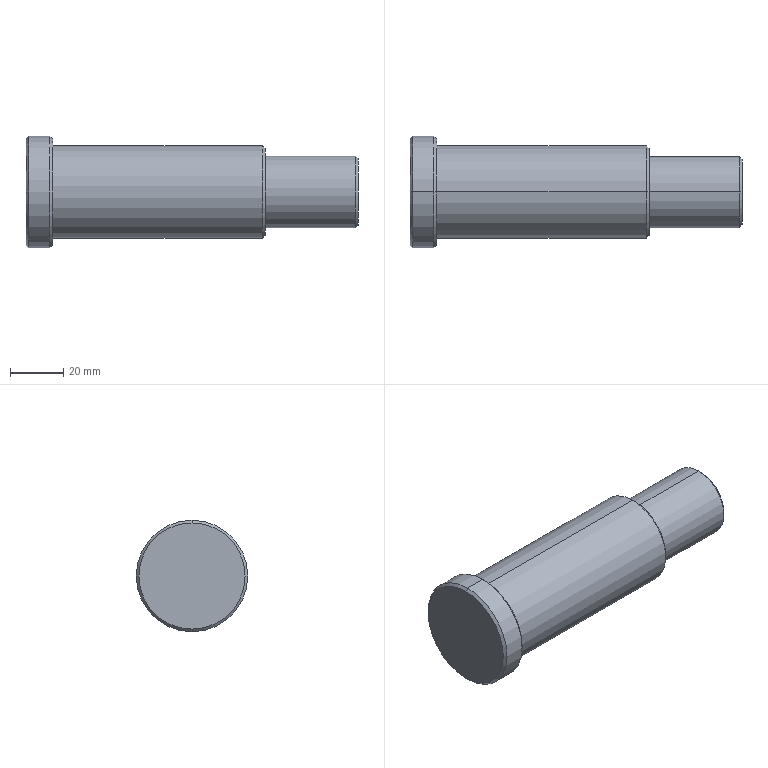Part | STEP file | BT2022003-01-09 Pin shaft C | 1 solid | 18 faces | box 125 x 42 x 42 mm | volume 110638 mm3 | cone 8 | cylinder 6 | plane 4 | commonest cylinder face diameters 27 x2 35 x2 42 x2
STEP:
#1=CARTESIAN_POINT('',(10.,0.,-20.));
#2=VERTEX_POINT('',#1);
#3=CARTESIAN_POINT('',(10.,0.,20.));
#4=VERTEX_POINT('',#3);
#5=CARTESIAN_POINT('',(10.,0.,0.));
#6=DIRECTION('',(1.,0.,0.));
#7=DIRECTION('',(0.,0.,1.));
#8=AXIS2_PLACEMENT_3D('',#5,#6,#7);
#9=CIRCLE('',#8,20.);
#10=EDGE_CURVE('',#2,#4,#9,.T.);
#11=ORIENTED_EDGE('',*,*,#10,.F.);
#12=CARTESIAN_POINT('',(9.,0.,-21.));
#13=VERTEX_POINT('',#12);
#14=CARTESIAN_POINT('',(9.,0.,-21.));
#15=DIRECTION('',(-0.7071,0.,-0.7071));
#16=VECTOR('',#15,1000.);
#17=LINE('',#14,#16);
#18=EDGE_CURVE('',#2,#13,#17,.T.);
#19=ORIENTED_EDGE('',*,*,#18,.T.);
#20=CARTESIAN_POINT('',(9.,0.,21.));
#21=VERTEX_POINT('',#20);
#22=CARTESIAN_POINT('',(9.,0.,0.));
#23=DIRECTION('',(-1.,0.,0.));
#24=DIRECTION('',(0.,0.,1.));
#25=AXIS2_PLACEMENT_3D('',#22,#23,#24);
#26=CIRCLE('',#25,21.);
#27=EDGE_CURVE('',#21,#13,#26,.T.);
#28=ORIENTED_EDGE('',*,*,#27,.F.);
#29=CARTESIAN_POINT('',(9.,0.,21.));
#30=DIRECTION('',(-0.7071,0.,0.7071));
#31=VECTOR('',#30,1000.);
#32=LINE('',#29,#31);
#33=EDGE_CURVE('',#4,#21,#32,.T.);
#34=ORIENTED_EDGE('',*,*,#33,.F.);
#35=EDGE_LOOP('',(#11,#19,#28,#34));
#36=FACE_OUTER_BOUND('',#35,.T.);
#37=CARTESIAN_POINT('',(9.,0.,0.));
#38=DIRECTION('',(-1.,0.,0.));
#39=DIRECTION('',(0.,0.,1.));
#40=AXIS2_PLACEMENT_3D('',#37,#38,#39);
#41=CONICAL_SURFACE('',#40,21.,0.7854);
#42=ADVANCED_FACE('',(#36),#41,.T.);
#43=CARTESIAN_POINT('',(0.,0.,20.));
#44=VERTEX_POINT('',#43);
#45=CARTESIAN_POINT('',(0.,0.,-20.));
#46=VERTEX_POINT('',#45);
#47=CARTESIAN_POINT('',(0.,0.,0.));
#48=DIRECTION('',(-1.,0.,0.));
#49=DIRECTION('',(0.,0.,-1.));
#50=AXIS2_PLACEMENT_3D('',#47,#48,#49);
#51=CIRCLE('',#50,20.);
#52=EDGE_CURVE('',#44,#46,#51,.T.);
#53=ORIENTED_EDGE('',*,*,#52,.F.);
#54=CARTESIAN_POINT('',(1.,0.,21.));
#55=VERTEX_POINT('',#54);
#56=CARTESIAN_POINT('',(0.,0.,20.));
#57=DIRECTION('',(0.7071,0.,0.7071));
#58=VECTOR('',#57,1000.);
#59=LINE('',#56,#58);
#60=EDGE_CURVE('',#44,#55,#59,.T.);
#61=ORIENTED_EDGE('',*,*,#60,.T.);
#62=CARTESIAN_POINT('',(1.,0.,-21.));
#63=VERTEX_POINT('',#62);
#64=CARTESIAN_POINT('',(1.,0.,0.));
#65=DIRECTION('',(1.,0.,0.));
#66=DIRECTION('',(0.,0.,-1.));
#67=AXIS2_PLACEMENT_3D('',#64,#65,#66);
#68=CIRCLE('',#67,21.);
#69=EDGE_CURVE('',#63,#55,#68,.T.);
#70=ORIENTED_EDGE('',*,*,#69,.F.);
#71=CARTESIAN_POINT('',(0.,0.,-20.));
#72=DIRECTION('',(0.7071,0.,-0.7071));
#73=VECTOR('',#72,1000.);
#74=LINE('',#71,#73);
#75=EDGE_CURVE('',#46,#63,#74,.T.);
#76=ORIENTED_EDGE('',*,*,#75,.F.);
#77=EDGE_LOOP('',(#53,#61,#70,#76));
#78=FACE_OUTER_BOUND('',#77,.T.);
#79=CARTESIAN_POINT('',(0.,0.,0.));
#80=DIRECTION('',(1.,0.,0.));
#81=DIRECTION('',(0.,0.,-1.));
#82=AXIS2_PLACEMENT_3D('',#79,#80,#81);
#83=CONICAL_SURFACE('',#82,20.,0.7854);
#84=ADVANCED_FACE('',(#78),#83,.T.);
#85=CARTESIAN_POINT('',(90.,0.,-16.5));
#86=VERTEX_POINT('',#85);
#87=CARTESIAN_POINT('',(90.,0.,16.5));
#88=VERTEX_POINT('',#87);
#89=CARTESIAN_POINT('',(90.,0.,0.));
#90=DIRECTION('',(1.,0.,0.));
#91=DIRECTION('',(0.,0.,1.));
#92=AXIS2_PLACEMENT_3D('',#89,#90,#91);
#93=CIRCLE('',#92,16.5);
#94=EDGE_CURVE('',#86,#88,#93,.T.);
#95=ORIENTED_EDGE('',*,*,#94,.F.);
#96=CARTESIAN_POINT('',(89.,0.,-17.5));
#97=VERTEX_POINT('',#96);
#98=CARTESIAN_POINT('',(89.,0.,-17.5));
#99=DIRECTION('',(-0.7071,0.,-0.7071));
#100=VECTOR('',#99,1000.);
#101=LINE('',#98,#100);
#102=EDGE_CURVE('',#86,#97,#101,.T.);
#103=ORIENTED_EDGE('',*,*,#102,.T.);
#104=CARTESIAN_POINT('',(89.,0.,17.5));
#105=VERTEX_POINT('',#104);
#106=CARTESIAN_POINT('',(89.,0.,0.));
#107=DIRECTION('',(-1.,0.,0.));
#108=DIRECTION('',(0.,0.,1.));
#109=AXIS2_PLACEMENT_3D('',#106,#107,#108);
#110=CIRCLE('',#109,17.5);
#111=EDGE_CURVE('',#105,#97,#110,.T.);
#112=ORIENTED_EDGE('',*,*,#111,.F.);
#113=CARTESIAN_POINT('',(89.,0.,17.5));
#114=DIRECTION('',(-0.7071,0.,0.7071));
#115=VECTOR('',#114,1000.);
#116=LINE('',#113,#115);
#117=EDGE_CURVE('',#88,#105,#116,.T.);
#118=ORIENTED_EDGE('',*,*,#117,.F.);
#119=EDGE_LOOP('',(#95,#103,#112,#118));
#120=FACE_OUTER_BOUND('',#119,.T.);
#121=CARTESIAN_POINT('',(89.,0.,0.));
#122=DIRECTION('',(-1.,0.,0.));
#123=DIRECTION('',(0.,0.,1.));
#124=AXIS2_PLACEMENT_3D('',#121,#122,#123);
#125=CONICAL_SURFACE('',#124,17.5,0.7854);
#126=ADVANCED_FACE('',(#120),#125,.T.);
#127=CARTESIAN_POINT('',(125.,0.,-12.5));
#128=VERTEX_POINT('',#127);
#129=CARTESIAN_POINT('',(125.,0.,12.5));
#130=VERTEX_POINT('',#129);
#131=CARTESIAN_POINT('',(125.,0.,0.));
#132=DIRECTION('',(1.,0.,0.));
#133=DIRECTION('',(0.,0.,1.));
#134=AXIS2_PLACEMENT_3D('',#131,#132,#133);
#135=CIRCLE('',#134,12.5);
#136=EDGE_CURVE('',#128,#130,#135,.T.);
#137=ORIENTED_EDGE('',*,*,#136,.F.);
#138=CARTESIAN_POINT('',(124.,0.,-13.5));
#139=VERTEX_POINT('',#138);
#140=CARTESIAN_POINT('',(124.,0.,-13.5));
#141=DIRECTION('',(-0.7071,0.,-0.7071));
#142=VECTOR('',#141,1000.);
#143=LINE('',#140,#142);
#144=EDGE_CURVE('',#128,#139,#143,.T.);
#145=ORIENTED_EDGE('',*,*,#144,.T.);
#146=CARTESIAN_POINT('',(124.,0.,13.5));
#147=VERTEX_POINT('',#146);
#148=CARTESIAN_POINT('',(124.,0.,0.));
#149=DIRECTION('',(-1.,0.,0.));
#150=DIRECTION('',(0.,0.,1.));
#151=AXIS2_PLACEMENT_3D('',#148,#149,#150);
#152=CIRCLE('',#151,13.5);
#153=EDGE_CURVE('',#147,#139,#152,.T.);
#154=ORIENTED_EDGE('',*,*,#153,.F.);
#155=CARTESIAN_POINT('',(124.,0.,13.5));
#156=DIRECTION('',(-0.7071,0.,0.7071));
#157=VECTOR('',#156,1000.);
#158=LINE('',#155,#157);
#159=EDGE_CURVE('',#130,#147,#158,.T.);
#160=ORIENTED_EDGE('',*,*,#159,.F.);
#161=EDGE_LOOP('',(#137,#145,#154,#160));
#162=FACE_OUTER_BOUND('',#161,.T.);
#163=CARTESIAN_POINT('',(124.,0.,0.));
#164=DIRECTION('',(-1.,0.,0.));
#165=DIRECTION('',(0.,0.,1.));
#166=AXIS2_PLACEMENT_3D('',#163,#164,#165);
#167=CONICAL_SURFACE('',#166,13.5,0.7854);
#168=ADVANCED_FACE('',(#162),#167,.T.);
#169=ORIENTED_EDGE('',*,*,#153,.T.);
#170=CARTESIAN_POINT('',(90.,0.,-13.5));
#171=VERTEX_POINT('',#170);
#172=CARTESIAN_POINT('',(0.,0.,-13.5));
#173=DIRECTION('',(-1.,0.,0.));
#174=VECTOR('',#173,1000.);
#175=LINE('',#172,#174);
#176=EDGE_CURVE('',#139,#171,#175,.T.);
#177=ORIENTED_EDGE('',*,*,#176,.T.);
#178=CARTESIAN_POINT('',(90.,0.,13.5));
#179=VERTEX_POINT('',#178);
#180=CARTESIAN_POINT('',(90.,0.,0.));
#181=DIRECTION('',(-1.,0.,0.));
#182=DIRECTION('',(0.,0.,1.));
#183=AXIS2_PLACEMENT_3D('',#180,#181,#182);
#184=CIRCLE('',#183,13.5);
#185=EDGE_CURVE('',#179,#171,#184,.T.);
#186=ORIENTED_EDGE('',*,*,#185,.F.);
#187=CARTESIAN_POINT('',(0.,0.,13.5));
#188=DIRECTION('',(-1.,0.,0.));
#189=VECTOR('',#188,1000.);
#190=LINE('',#187,#189);
#191=EDGE_CURVE('',#147,#179,#190,.T.);
#192=ORIENTED_EDGE('',*,*,#191,.F.);
#193=EDGE_LOOP('',(#169,#177,#186,#192));
#194=FACE_OUTER_BOUND('',#193,.T.);
#195=CARTESIAN_POINT('',(0.,0.,0.));
#196=DIRECTION('',(-1.,0.,0.));
#197=DIRECTION('',(0.,0.,1.));
#198=AXIS2_PLACEMENT_3D('',#195,#196,#197);
#199=CYLINDRICAL_SURFACE('',#198,13.5);
#200=ADVANCED_FACE('',(#194),#199,.T.);
#201=ORIENTED_EDGE('',*,*,#111,.T.);
#202=CARTESIAN_POINT('',(10.,0.,-17.5));
#203=VERTEX_POINT('',#202);
#204=CARTESIAN_POINT('',(0.,0.,-17.5));
#205=DIRECTION('',(-1.,0.,0.));
#206=VECTOR('',#205,1000.);
#207=LINE('',#204,#206);
#208=EDGE_CURVE('',#97,#203,#207,.T.);
#209=ORIENTED_EDGE('',*,*,#208,.T.);
#210=CARTESIAN_POINT('',(10.,0.,17.5));
#211=VERTEX_POINT('',#210);
#212=CARTESIAN_POINT('',(10.,0.,0.));
#213=DIRECTION('',(-1.,0.,0.));
#214=DIRECTION('',(0.,0.,1.));
#215=AXIS2_PLACEMENT_3D('',#212,#213,#214);
#216=CIRCLE('',#215,17.5);
#217=EDGE_CURVE('',#211,#203,#216,.T.);
#218=ORIENTED_EDGE('',*,*,#217,.F.);
#219=CARTESIAN_POINT('',(0.,0.,17.5));
#220=DIRECTION('',(-1.,0.,0.));
#221=VECTOR('',#220,1000.);
#222=LINE('',#219,#221);
#223=EDGE_CURVE('',#105,#211,#222,.T.);
#224=ORIENTED_EDGE('',*,*,#223,.F.);
#225=EDGE_LOOP('',(#201,#209,#218,#224));
#226=FACE_OUTER_BOUND('',#225,.T.);
#227=CARTESIAN_POINT('',(0.,0.,0.));
#228=DIRECTION('',(-1.,0.,0.));
#229=DIRECTION('',(0.,0.,1.));
#230=AXIS2_PLACEMENT_3D('',#227,#228,#229);
#231=CYLINDRICAL_SURFACE('',#230,17.5);
#232=ADVANCED_FACE('',(#226),#231,.T.);
#233=ORIENTED_EDGE('',*,*,#27,.T.);
#234=CARTESIAN_POINT('',(0.,0.,-21.));
#235=DIRECTION('',(-1.,0.,0.));
#236=VECTOR('',#235,1000.);
#237=LINE('',#234,#236);
#238=EDGE_CURVE('',#13,#63,#237,.T.);
#239=ORIENTED_EDGE('',*,*,#238,.T.);
#240=ORIENTED_EDGE('',*,*,#69,.T.);
#241=CARTESIAN_POINT('',(0.,0.,21.));
#242=DIRECTION('',(-1.,0.,0.));
#243=VECTOR('',#242,1000.);
#244=LINE('',#241,#243);
#245=EDGE_CURVE('',#21,#55,#244,.T.);
#246=ORIENTED_EDGE('',*,*,#245,.F.);
#247=EDGE_LOOP('',(#233,#239,#240,#246));
#248=FACE_OUTER_BOUND('',#247,.T.);
#249=CARTESIAN_POINT('',(0.,0.,0.));
#250=DIRECTION('',(-1.,0.,0.));
#251=DIRECTION('',(0.,0.,1.));
#252=AXIS2_PLACEMENT_3D('',#249,#250,#251);
#253=CYLINDRICAL_SURFACE('',#252,21.);
#254=ADVANCED_FACE('',(#248),#253,.T.);
#255=CARTESIAN_POINT('',(0.,0.,0.));
#256=DIRECTION('',(-1.,0.,0.));
#257=DIRECTION('',(0.,0.,-1.));
#258=AXIS2_PLACEMENT_3D('',#255,#256,#257);
#259=CIRCLE('',#258,20.);
#260=EDGE_CURVE('',#46,#44,#259,.T.);
#261=ORIENTED_EDGE('',*,*,#260,.T.);
#262=ORIENTED_EDGE('',*,*,#52,.T.);
#263=EDGE_LOOP('',(#261,#262));
#264=FACE_OUTER_BOUND('',#263,.T.);
#265=CARTESIAN_POINT('',(0.,0.,0.));
#266=DIRECTION('',(1.,0.,0.));
#267=DIRECTION('',(0.,0.,-1.));
#268=AXIS2_PLACEMENT_3D('',#265,#266,#267);
#269=PLANE('',#268);
#270=ADVANCED_FACE('',(#264),#269,.F.);
#271=ORIENTED_EDGE('',*,*,#238,.F.);
#272=CARTESIAN_POINT('',(9.,0.,0.));
#273=DIRECTION('',(-1.,0.,0.));
#274=DIRECTION('',(0.,0.,1.));
#275=AXIS2_PLACEMENT_3D('',#272,#273,#274);
#276=CIRCLE('',#275,21.);
#277=EDGE_CURVE('',#13,#21,#276,.T.);
#278=ORIENTED_EDGE('',*,*,#277,.T.);
#279=ORIENTED_EDGE('',*,*,#245,.T.);
#280=CARTESIAN_POINT('',(1.,0.,0.));
#281=DIRECTION('',(1.,0.,0.));
#282=DIRECTION('',(0.,0.,-1.));
#283=AXIS2_PLACEMENT_3D('',#280,#281,#282);
#284=CIRCLE('',#283,21.);
#285=EDGE_CURVE('',#55,#63,#284,.T.);
#286=ORIENTED_EDGE('',*,*,#285,.T.);
#287=EDGE_LOOP('',(#271,#278,#279,#286));
#288=FACE_OUTER_BOUND('',#287,.T.);
#289=CARTESIAN_POINT('',(0.,0.,0.));
#290=DIRECTION('',(-1.,0.,0.));
#291=DIRECTION('',(0.,0.,1.));
#292=AXIS2_PLACEMENT_3D('',#289,#290,#291);
#293=CYLINDRICAL_SURFACE('',#292,21.);
#294=ADVANCED_FACE('',(#288),#293,.T.);
#295=CARTESIAN_POINT('',(10.,0.,0.));
#296=DIRECTION('',(1.,0.,0.));
#297=DIRECTION('',(0.,0.,1.));
#298=AXIS2_PLACEMENT_3D('',#295,#296,#297);
#299=CIRCLE('',#298,20.);
#300=EDGE_CURVE('',#4,#2,#299,.T.);
#301=ORIENTED_EDGE('',*,*,#300,.T.);
#302=ORIENTED_EDGE('',*,*,#10,.T.);
#303=EDGE_LOOP('',(#301,#302));
#304=FACE_OUTER_BOUND('',#303,.T.);
#305=ORIENTED_EDGE('',*,*,#217,.T.);
#306=CARTESIAN_POINT('',(10.,0.,0.));
#307=DIRECTION('',(-1.,0.,0.));
#308=DIRECTION('',(0.,0.,1.));
#309=AXIS2_PLACEMENT_3D('',#306,#307,#308);
#310=CIRCLE('',#309,17.5);
#311=EDGE_CURVE('',#203,#211,#310,.T.);
#312=ORIENTED_EDGE('',*,*,#311,.T.);
#313=EDGE_LOOP('',(#305,#312));
#314=FACE_BOUND('',#313,.T.);
#315=CARTESIAN_POINT('',(10.,21.,0.));
#316=DIRECTION('',(-1.,0.,0.));
#317=DIRECTION('',(0.,0.,1.));
#318=AXIS2_PLACEMENT_3D('',#315,#316,#317);
#319=PLANE('',#318);
#320=ADVANCED_FACE('',(#304,#314),#319,.F.);
#321=ORIENTED_EDGE('',*,*,#208,.F.);
#322=CARTESIAN_POINT('',(89.,0.,0.));
#323=DIRECTION('',(-1.,0.,0.));
#324=DIRECTION('',(0.,0.,1.));
#325=AXIS2_PLACEMENT_3D('',#322,#323,#324);
#326=CIRCLE('',#325,17.5);
#327=EDGE_CURVE('',#97,#105,#326,.T.);
#328=ORIENTED_EDGE('',*,*,#327,.T.);
#329=ORIENTED_EDGE('',*,*,#223,.T.);
#330=ORIENTED_EDGE('',*,*,#311,.F.);
#331=EDGE_LOOP('',(#321,#328,#329,#330));
#332=FACE_OUTER_BOUND('',#331,.T.);
#333=CARTESIAN_POINT('',(0.,0.,0.));
#334=DIRECTION('',(-1.,0.,0.));
#335=DIRECTION('',(0.,0.,1.));
#336=AXIS2_PLACEMENT_3D('',#333,#334,#335);
#337=CYLINDRICAL_SURFACE('',#336,17.5);
#338=ADVANCED_FACE('',(#332),#337,.T.);
#339=CARTESIAN_POINT('',(90.,0.,0.));
#340=DIRECTION('',(1.,0.,0.));
#341=DIRECTION('',(0.,0.,1.));
#342=AXIS2_PLACEMENT_3D('',#339,#340,#341);
#343=CIRCLE('',#342,16.5);
#344=EDGE_CURVE('',#88,#86,#343,.T.);
#345=ORIENTED_EDGE('',*,*,#344,.T.);
#346=ORIENTED_EDGE('',*,*,#94,.T.);
#347=EDGE_LOOP('',(#345,#346));
#348=FACE_OUTER_BOUND('',#347,.T.);
#349=ORIENTED_EDGE('',*,*,#185,.T.);
#350=CARTESIAN_POINT('',(90.,0.,0.));
#351=DIRECTION('',(-1.,0.,0.));
#352=DIRECTION('',(0.,0.,1.));
#353=AXIS2_PLACEMENT_3D('',#350,#351,#352);
#354=CIRCLE('',#353,13.5);
#355=EDGE_CURVE('',#171,#179,#354,.T.);
#356=ORIENTED_EDGE('',*,*,#355,.T.);
#357=EDGE_LOOP('',(#349,#356));
#358=FACE_BOUND('',#357,.T.);
#359=CARTESIAN_POINT('',(90.,17.5,0.));
#360=DIRECTION('',(-1.,0.,0.));
#361=DIRECTION('',(0.,0.,1.));
#362=AXIS2_PLACEMENT_3D('',#359,#360,#361);
#363=PLANE('',#362);
#364=ADVANCED_FACE('',(#348,#358),#363,.F.);
#365=ORIENTED_EDGE('',*,*,#176,.F.);
#366=CARTESIAN_POINT('',(124.,0.,0.));
#367=DIRECTION('',(-1.,0.,0.));
#368=DIRECTION('',(0.,0.,1.));
#369=AXIS2_PLACEMENT_3D('',#366,#367,#368);
#370=CIRCLE('',#369,13.5);
#371=EDGE_CURVE('',#139,#147,#370,.T.);
#372=ORIENTED_EDGE('',*,*,#371,.T.);
#373=ORIENTED_EDGE('',*,*,#191,.T.);
#374=ORIENTED_EDGE('',*,*,#355,.F.);
#375=EDGE_LOOP('',(#365,#372,#373,#374));
#376=FACE_OUTER_BOUND('',#375,.T.);
#377=CARTESIAN_POINT('',(0.,0.,0.));
#378=DIRECTION('',(-1.,0.,0.));
#379=DIRECTION('',(0.,0.,1.));
#380=AXIS2_PLACEMENT_3D('',#377,#378,#379);
#381=CYLINDRICAL_SURFACE('',#380,13.5);
#382=ADVANCED_FACE('',(#376),#381,.T.);
#383=CARTESIAN_POINT('',(125.,0.,0.));
#384=DIRECTION('',(1.,0.,0.));
#385=DIRECTION('',(0.,0.,1.));
#386=AXIS2_PLACEMENT_3D('',#383,#384,#385);
#387=CIRCLE('',#386,12.5);
#388=EDGE_CURVE('',#130,#128,#387,.T.);
#389=ORIENTED_EDGE('',*,*,#388,.T.);
#390=ORIENTED_EDGE('',*,*,#136,.T.);
#391=EDGE_LOOP('',(#389,#390));
#392=FACE_OUTER_BOUND('',#391,.T.);
#393=CARTESIAN_POINT('',(125.,13.5,0.));
#394=DIRECTION('',(-1.,0.,0.));
#395=DIRECTION('',(0.,0.,1.));
#396=AXIS2_PLACEMENT_3D('',#393,#394,#395);
#397=PLANE('',#396);
#398=ADVANCED_FACE('',(#392),#397,.F.);
#399=ORIENTED_EDGE('',*,*,#144,.F.);
#400=ORIENTED_EDGE('',*,*,#388,.F.);
#401=ORIENTED_EDGE('',*,*,#159,.T.);
#402=ORIENTED_EDGE('',*,*,#371,.F.);
#403=EDGE_LOOP('',(#399,#400,#401,#402));
#404=FACE_OUTER_BOUND('',#403,.T.);
#405=CARTESIAN_POINT('',(124.,0.,0.));
#406=DIRECTION('',(-1.,0.,0.));
#407=DIRECTION('',(0.,0.,1.));
#408=AXIS2_PLACEMENT_3D('',#405,#406,#407);
#409=CONICAL_SURFACE('',#408,13.5,0.7854);
#410=ADVANCED_FACE('',(#404),#409,.T.);
#411=ORIENTED_EDGE('',*,*,#102,.F.);
#412=ORIENTED_EDGE('',*,*,#344,.F.);
#413=ORIENTED_EDGE('',*,*,#117,.T.);
#414=ORIENTED_EDGE('',*,*,#327,.F.);
#415=EDGE_LOOP('',(#411,#412,#413,#414));
#416=FACE_OUTER_BOUND('',#415,.T.);
#417=CARTESIAN_POINT('',(89.,0.,0.));
#418=DIRECTION('',(-1.,0.,0.));
#419=DIRECTION('',(0.,0.,1.));
#420=AXIS2_PLACEMENT_3D('',#417,#418,#419);
#421=CONICAL_SURFACE('',#420,17.5,0.7854);
#422=ADVANCED_FACE('',(#416),#421,.T.);
#423=ORIENTED_EDGE('',*,*,#60,.F.);
#424=ORIENTED_EDGE('',*,*,#260,.F.);
#425=ORIENTED_EDGE('',*,*,#75,.T.);
#426=ORIENTED_EDGE('',*,*,#285,.F.);
#427=EDGE_LOOP('',(#423,#424,#425,#426));
#428=FACE_OUTER_BOUND('',#427,.T.);
#429=CARTESIAN_POINT('',(0.,0.,0.));
#430=DIRECTION('',(1.,0.,0.));
#431=DIRECTION('',(0.,0.,-1.));
#432=AXIS2_PLACEMENT_3D('',#429,#430,#431);
#433=CONICAL_SURFACE('',#432,20.,0.7854);
#434=ADVANCED_FACE('',(#428),#433,.T.);
#435=ORIENTED_EDGE('',*,*,#18,.F.);
#436=ORIENTED_EDGE('',*,*,#300,.F.);
#437=ORIENTED_EDGE('',*,*,#33,.T.);
#438=ORIENTED_EDGE('',*,*,#277,.F.);
#439=EDGE_LOOP('',(#435,#436,#437,#438));
#440=FACE_OUTER_BOUND('',#439,.T.);
#441=CARTESIAN_POINT('',(9.,0.,0.));
#442=DIRECTION('',(-1.,0.,0.));
#443=DIRECTION('',(0.,0.,1.));
#444=AXIS2_PLACEMENT_3D('',#441,#442,#443);
#445=CONICAL_SURFACE('',#444,21.,0.7854);
#446=ADVANCED_FACE('',(#440),#445,.T.);
#447=CLOSED_SHELL('',(#42,#84,#126,#168,#200,#232,#254,#270,#294,#320,#338,#364,#382,#398,#410,#422,#434,#446));
#448=MANIFOLD_SOLID_BREP('',#447);
#449=CARTESIAN_POINT('',(0.,0.,0.));
#450=DIRECTION('',(0.,0.,1.));
#451=DIRECTION('',(1.,0.,0.));
#452=AXIS2_PLACEMENT_3D('',#449,#450,#451);
#453=(LENGTH_UNIT()NAMED_UNIT(*)SI_UNIT(.MILLI.,.METRE.));
#454=UNCERTAINTY_MEASURE_WITH_UNIT(LENGTH_MEASURE(0.00001),#453,'','');
#455=(NAMED_UNIT(*)PLANE_ANGLE_UNIT()SI_UNIT($,.RADIAN.));
#456=(NAMED_UNIT(*)SI_UNIT($,.STERADIAN.)SOLID_ANGLE_UNIT());
#457=(GEOMETRIC_REPRESENTATION_CONTEXT(3)GLOBAL_UNCERTAINTY_ASSIGNED_CONTEXT((#454))GLOBAL_UNIT_ASSIGNED_CONTEXT((#453,#455,#456))REPRESENTATION_CONTEXT('',''));
#458=ADVANCED_BREP_SHAPE_REPRESENTATION('',(#448,#452),#457);